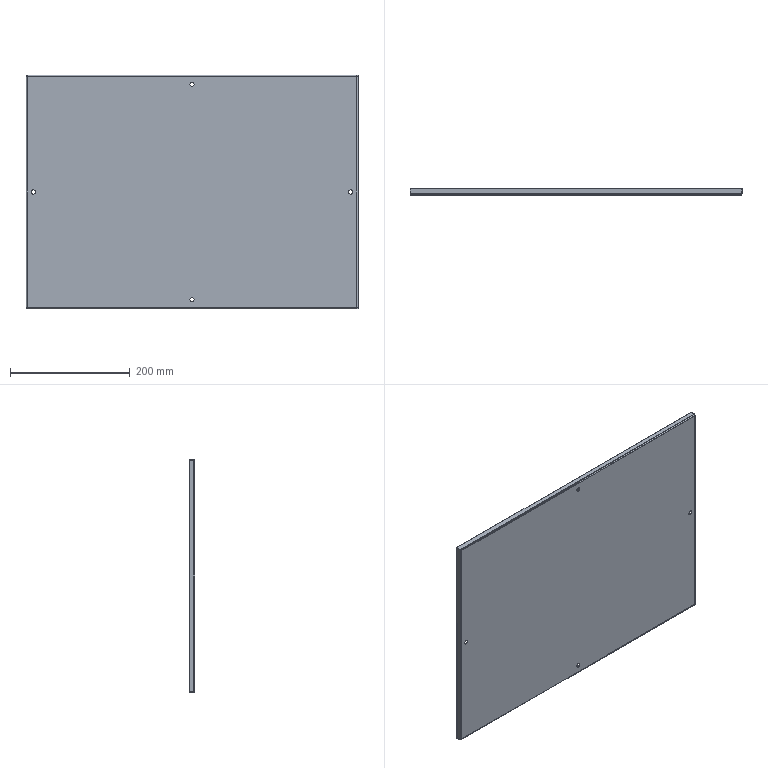Part | STEP file | Large bent plate rear cover | 1 solid | 54 faces | box 555 x 10 x 390 mm | volume 277878 mm3 | plane 38 | cylinder 16 | commonest cylinder face diameters 7 x8 2 x4 4.4 x4